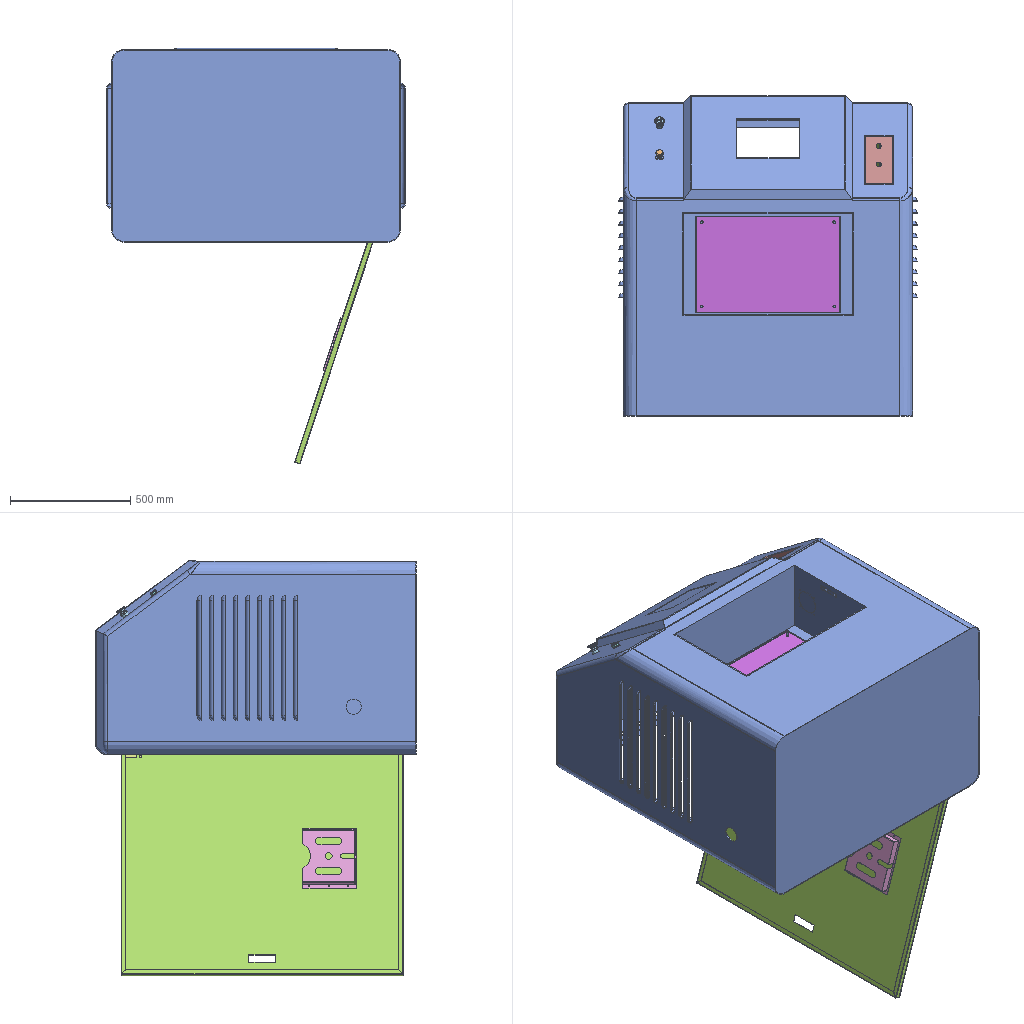Assembly | SolidWorks | 7 different items | 7 placed | box 1240 x 1330 x 1726 mm
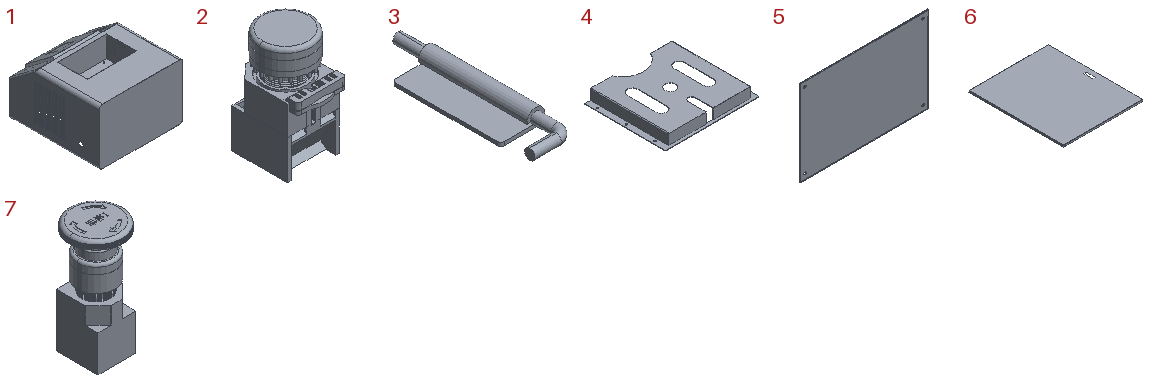Parts list (item | quantity | size | volume | features):
1 | x1 | 1240 x 1330 x 806 mm | 19071542 mm3 | features ICE 18, Cut 7, Fillet 4, Chamfer 2, MirrorPattern 2, Shell 2, Extrusion 1, LPattern 1
2 | x1 | 29.7 x 39.925 x 61.4 mm | 43497 mm3 | features ICE 36, Fillet 3, MirrorPattern 3, Extrusion 1, Helix 1, Revolution 1, SweepCut 1
3 | x1 | 25 x 98 x 10 mm | 8135 mm3 | features Extrusion 1, Fillet 1, Sweep 1
4 | x1 | 261 x 226 x 30 mm | 80128 mm3 | features ICE 4, Fillet 2, Extrusion 1, HoleWzd 1, SketchPattern 1
5 | x1 | 600 x 4 x 400 mm | 487208 mm3 | features Cut 1, Extrusion 1, Shell 1
6 | x1 | 982 x 1182 x 24 mm | 1971875 mm3 | features Cut 2, EdgeFlange 2, ICE 2, Chamfer 1, FlatPattern 1, SMBaseFlange 1, SheetMetal 1
7 | x1 | 40.499 x 40.499 x 87.5 mm | 63476 mm3 | features ICE 10, Fillet 4, CirPattern 2, RevCut 2, Extrusion 1, LPattern 1
Mates (type | each side: item.copy, entity, surface, feature):
Concentric | 1.1 face cylinder Cut-Extrude1 | 6.1 face cylinder Boss-Extrude2
Coincident | 6.1 face plane Base-Flange1 | 4.1 face plane Boss-Extrude2
DistanceDim | 4.1 face plane Boss-Extrude2 | 6.1 face plane Edge-Flange1
DistanceDim | 6.1 face plane Edge-Flange1 | 4.1 face plane Boss-Extrude2
Coincident | 1.1 face plane Boss-Extrude3 | 6.1 face plane Boss-Extrude1
Parallel | 1.1 face plane Chamfer1 | 7.1 face plane Extrude6
Concentric | 1.1 edge | 7.1 face cylinder Extrude3
Coincident | 1.1 face plane Chamfer1 | 7.1 face plane Extrude3
Concentric | 1.1 edge | 2.1 face cylinder Revolve1
Coincident | 1.1 face plane Chamfer1 | 2.1 face plane Boss-Extrude6
Concentric | 6.1 face cylinder Cut-Extrude2 | 3.1 face cylinder Sweep1
Parallel | 6.1 face plane Edge-Flange2 | 3.1 face plane Boss-Extrude1
Coincident | 6.1 face plane Edge-Flange1 | 3.1 face plane Boss-Extrude1
Parallel | 1.1 face plane Boss-Extrude9 | 5.1 face plane Boss-Extrude1
Coincident | 1.1 face plane Boss-Extrude9 | 5.1 face plane Boss-Extrude1
Symmetric | 1.1 face plane Cut-Extrude10 | 1.1 face plane Cut-Extrude10 | 5.1 plane | 2 times